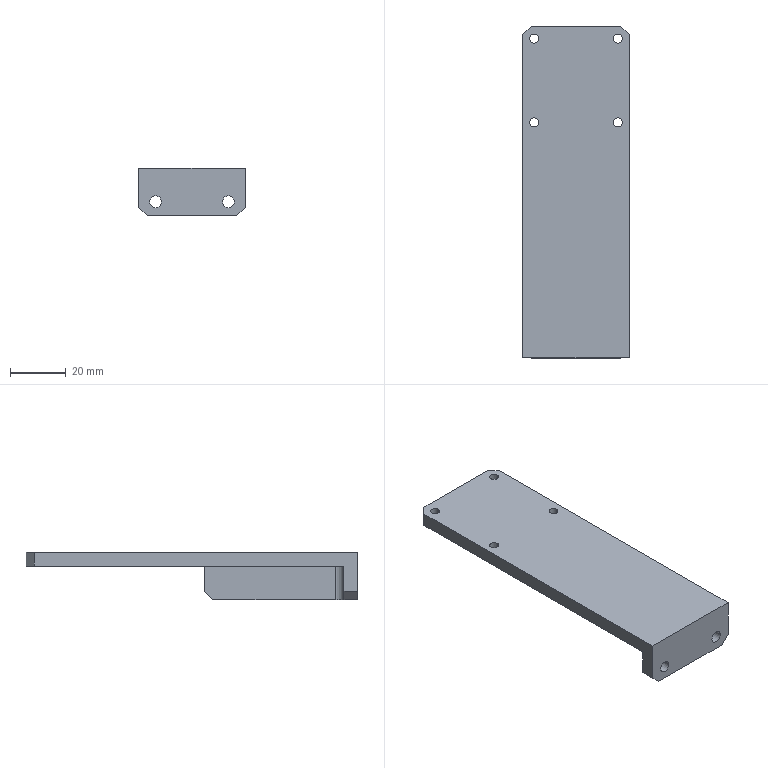NC program | NX | posted with a generic post | part box 38.1 x 118.8 x 17 mm
Whole program:
N10 G17 G21 G94 G90
(FLOOR_WALL_COPY , TOOL : D80)
N12 T19 M6
N14 G54
N16 G17 G0 G90 X-108.4 Y0. S6500 M3
N18 G43 Z30. H19
N20 Z3.
N22 G94 G1 Z0. F1500.
N24 X-103.4
N26 X103.4
N28 X108.4
N30 Z3.
N32 G0 Z30.
N34 M5
(DRILLING_COPY_1 , TOOL : D6A45)
N36 T01 M6
N38 G54
N40 G17 G0 G90 X24.9 Y15. S5000 M3
N42 G43 Z30. H1
N44 G94 G81 G98 Z-1. F350. R3.
N46 X54.9
N48 Y-15.
N50 X24.9
N52 G80
N54 G0 X24.9 Y-15. Z30.
N56 M5
(DRILLING_COPY_1_COPY_1 , TOOL : 3.2ZT)
N58 T03 M6
N60 G54
N62 G17 G0 G90 X24.9 Y15. S2000 M3
N64 G43 Z30. H3
N66 G94 G83 G98 Z-7.461 F180. Q2. R3.
N68 X54.9
N70 Y-15.
N72 X24.9
N74 G80
N76 G0 X24.9 Y-15. Z30.
N78 M5
(ADAPTIVE_MILLING , TOOL : D10)
N80 T15 M6
N82 G54
N84 G17 G0 G90 X0.038 Y30.759 S9500 M3
N86 G43 Z30. H15
N88 Z-14.
N90 G94 G1 Z-17. F1000.
N92 X-0.241 Y29.978 F3000.
N94 X-0.498 Y29.19
N96 G3 X0.038 Y28.112 R1.017
N98 X3.102 Y27.351 R8.28
N100 X12.969 Y27.069 R111.643
N102 G1 X15.219 Y27.064
N104 X19.094 Y27.061
N106 X32.719 Y27.06
N108 X60.344
N110 X60.594 Y27.055
N112 X60.719 Y27.046
N114 G2 X64.982 Y24.28 R5.993
N116 X66.931 Y18.661 R13.127
N118 X67.368 Y9.428 R74.333
N120 G1 X67.376 Y8.053
N122 X67.382 Y6.178
N124 X67.386 Y3.428
N126 X67.388 Y-2.072
N128 Y-20.072
N130 X67.386 Y-20.197
N132 G2 X64.882 Y-24.473 R5.736
N134 X59.312 Y-26.542 R12.477
N136 X50.457 Y-27.012 R65.248
N138 G1 X49.082 Y-27.022
N140 X47.582 Y-27.029
N142 X45.457 Y-27.034
N144 X42.082 Y-27.037
N146 X32.582 Y-27.038
N148 X-60.418
N150 G2 X-64.585 Y-24.819 R5.588
N152 X-66.807 Y-19.448 R11.664
N154 X-67.341 Y-11.85 R49.288
N156 G1 X-67.353 Y-10.975
N158 X-67.363 Y-9.975
N160 X-67.372 Y-8.725
N162 X-67.379 Y-7.1
N164 X-67.384 Y-4.85
N166 X-67.387 Y-1.1
N168 X-67.388 Y10.9
N170 Y20.025
N172 X-67.387 Y20.15
N174 X-67.382 Y20.275
N176 X-67.374 Y20.399
N178 G2 X-64.602 Y24.658 R5.958
N180 X-58.977 Y26.588 R13.219
N182 X-50.368 Y27.013 R69.988
N184 G1 X-49.118 Y27.021
N186 X-47.493 Y27.029
N188 X-45.243 Y27.034
N190 X-41.618 Y27.037
N192 X-30.618 Y27.038
N194 X-3.743
N196 G2 X1.729 Y26.518 R60.908
N198 G3 X13.217 Y26.09 R124.4
N200 G1 X14.967 Y26.082
N202 X17.092 Y26.077
N204 X20.467 Y26.073
N206 X27.217 Y26.071
N208 X57.217 Y26.07
N210 X57.467 Y26.068
N212 G2 X63.753 Y22.33 R7.674
N214 X65.873 Y15.977 R15.701
N216 X66.349 Y6.37 R79.223
N218 G1 X66.358 Y5.12
N220 X66.366 Y3.495
N222 X66.372 Y1.245
N224 X66.375 Y-2.13
N226 X66.377 Y-9.63
N228 Y-17.005
N230 G2 X62.752 Y-23.349 R7.595
N232 X56.539 Y-25.491 R15.229
N234 X46.81 Y-25.998 R75.518
N236 G1 X45.435 Y-26.008
N238 X43.935 Y-26.015
N240 X41.81 Y-26.021
N242 X38.81 Y-26.025
N244 X32.435 Y-26.027
N246 X-57.315
N248 G2 X-63.675 Y-22.429 R7.603
N250 X-65.867 Y-15.974 R15.279
N252 X-66.345 Y-6.743 R74.856
N254 G1 X-66.355 Y-5.618
N256 X-66.363 Y-4.118
N258 X-66.369 Y-2.243
N260 X-66.374 Y0.507
N262 X-66.377 Y5.382
N264 Y16.882
N266 G2 X-62.743 Y23.346 R7.598
N268 X-56.283 Y25.527 R15.448
N270 X-46.926 Y25.997 R78.149
N272 G1 X-45.676 Y26.007
N274 X-44.301 Y26.014
N276 X-42.551 Y26.02
N278 X-39.801 Y26.024
N280 X-34.801 Y26.027
N282 X-6.176
N284 G2 X1.431 Y25.542 R94.226
N286 G3 X16.545 Y25.095 R192.713
N288 G1 X18.795 Y25.088
N290 X22.045 Y25.084
N292 X27.92 Y25.082
N294 X54.295 Y25.081
N296 X54.67 Y25.079
N298 X54.92 Y25.076
N300 G2 X62.852 Y20.266 R8.971
N302 G3 X63.887 Y18.561 R8.559
N304 G2 X64.702 Y15.593 R8.871
N306 X65.319 Y5.495 R74.892
N308 G1 X65.332 Y4.37
N310 X65.341 Y3.246
N312 X65.35 Y1.746
N314 X65.357 Y-0.129
N316 X65.362 Y-2.754
N318 X65.365 Y-7.004
N320 G2 X65.328 Y-15.378 R300.794
N322 X60.743 Y-22.413 R8.874
N324 G3 X58.911 Y-23.537 R10.258
N326 G2 X55.944 Y-24.353 R8.925
N328 X45.47 Y-24.973 R78.124
N330 G1 X44.22 Y-24.986
N332 X42.97 Y-24.996
N334 X41.47 Y-25.003
N336 X39.345 Y-25.009
N338 X36.22 Y-25.014
N340 X30.345 Y-25.016
N342 X-54.655 Y-25.017
N344 X-55.03 Y-25.012
N346 X-55.155 Y-25.009
N348 X-55.404 Y-25.
N350 X-55.529 Y-24.993
N352 G2 X-58.795 Y-24.212 R11.41
N354 X-60.797 Y-23.998 R12.163
N356 X-63.887 Y-21.561 R5.458
N358 X-64.545 Y-19.084 R5.984
N360 X-65.342 Y-3.74 R126.963
N362 G1 X-65.351 Y-2.115
N364 X-65.358 Y0.01
N366 X-65.363 Y3.01
N368 X-65.366 Y8.01
N370 Y14.26
N372 X-65.363 Y14.635
N374 G2 X-64.572 Y18.401 R9.73
N376 X-64.348 Y20.447 R14.412
N378 X-61.911 Y23.537 R5.458
N380 X-59.434 Y24.195 R5.984
N382 X-44.84 Y24.986 R120.72
N384 G1 X-43.34 Y24.996
N386 X-41.465 Y25.005
N388 X-39.09 Y25.01
N390 X-35.465 Y25.015
N392 X-28.09 Y25.016
N394 X-7.84 Y25.017
N396 G2 X0.896 Y24.573 R122.606
N398 G3 X9.117 Y24.2 R216.611
N400 G1 X56.365
N402 X56.434 Y24.195
N404 G2 X60.014 Y22.713 R5.569
N406 G1 X60.066 Y22.667
N408 X63.017 Y19.716
N410 X63.063 Y19.664
N412 X63.443 Y19.168
N414 X63.676 Y18.872
N416 X63.887 Y18.561
N418 X64.348 Y17.447
N420 X64.384 Y17.314
N422 X64.545 Y16.084
N424 X64.55 Y16.015
N426 Y-16.015
N428 X64.545 Y-16.084
N430 G2 X63.063 Y-19.664 R5.569
N432 G1 X63.017 Y-19.716
N434 X60.066 Y-22.667
N436 X60.014 Y-22.713
N438 X59.617 Y-23.017
N440 X59.273 Y-23.289
N442 X58.911 Y-23.537
N444 X57.797 Y-23.998
N446 X57.664 Y-24.034
N448 X56.434 Y-24.195
N450 X56.365 Y-24.2
N452 X-58.885
N454 G2 X-62.03 Y-23.468 R6.018
N456 X-64.384 Y-20.314 R5.458
N458 G1 X-64.545 Y-19.084
N460 X-64.55 Y-19.015
N462 Y18.61
N464 G2 X-63.818 Y21.68 R5.969
N466 X-60.664 Y24.034 R5.458
N468 G1 X-59.434 Y24.195
N470 X-59.365 Y24.2
N472 X9.135
N474 G3 X10.132 Y25.05 R1.016
N476 G1 X10.383 Y26.621
N478 Z-14.
N480 G0 Z30.
N482 M5
(ZLEVEL_PROFILE_COPY_1_COPY_COPY_1 , TOOL : D10JING)
N484 T14 M6
N486 G54
N488 G17 G0 G90 X-61.022 Y25.859 S9500 M3
N490 G43 Z30. H14
N492 Z-16.
N494 G94 G1 Z-17. F1000.
N496 X-60.266 Y24.55
N498 G3 X-59.4 Y24.05 R1.
N500 G1 X56.4 F1200.
N502 G2 X59.936 Y22.586 R5.
N504 G1 X62.936 Y19.586
N506 G2 X64.4 Y16.05 R5.
N508 G1 Y-16.05
N510 G2 X62.936 Y-19.586 R5.
N512 G1 X59.936 Y-22.586
N514 G2 X56.4 Y-24.05 R5.
N516 G1 X-59.4
N518 G2 X-64.4 Y-19.05 R5.
N520 G1 Y19.05
N522 G2 X-59.4 Y24.05 R5.
N524 G3 X-58.534 Y24.55 R1.
N526 G1 X-57.668 Y26.05
N528 Z-16.
N530 G0 Z30.
N532 M5
(PLANAR_MILL_COPY_COPY_COPY_COPY_COPY_COPY_1_COPY_1 , TOOL : D6A45)
N534 T01 M6
N536 G54
N538 G17 G0 G90 X55.333 Y15.45 S9500 M3
N540 G43 Z30. H1
N542 Z0.5
N544 G94 G1 Z-1. F1250.
N546 G3 X54.9 Y15.7 R0.5
N548 X54.2 Y15. R0.7
N550 X54.9 Y15.7 R-0.7
N552 X54.467 Y15.45 R0.5
N554 G1 Z0.5
N556 G0 Z30.
N558 X25.333
N560 Z0.5
N562 G1 Z-1.
N564 G3 X24.9 Y15.7 R0.5
N566 X24.2 Y15. R0.7
N568 X24.9 Y15.7 R-0.7
N570 X24.467 Y15.45 R0.5
N572 G1 Z0.5
N574 G0 Z30.
N576 X-2.366 Y20.45
N578 Z0.5
N580 G1 Z-1.
N582 G3 X-1.5 Y19.95 R1.
N584 G1 X56.4
N586 G2 X57.036 Y19.686 R0.9
N588 G1 X60.036 Y16.686
N590 G2 X60.3 Y16.05 R0.9
N592 G1 Y-16.05
N594 G2 X60.036 Y-16.686 R0.9
N596 G1 X57.036 Y-19.686
N598 G2 X56.4 Y-19.95 R0.9
N600 G1 X-59.4
N602 G2 X-60.3 Y-19.05 R0.9
N604 G1 Y19.05
N606 G2 X-59.4 Y19.95 R0.9
N608 G1 X-1.5
N610 G3 X-0.634 Y20.45 R1.
N612 G1 Z0.5
N614 G0 Z30.
N616 X24.467 Y-15.45
N618 Z0.5
N620 G1 Z-1.
N622 G3 X24.9 Y-15.7 R0.5
N624 X25.6 Y-15. R0.7
N626 X24.9 Y-15.7 R-0.7
N628 X25.333 Y-15.45 R0.5
N630 G1 Z0.5
N632 G0 Z30.
N634 X54.467
N636 Z0.5
N638 G1 Z-1.
N640 G3 X54.9 Y-15.7 R0.5
N642 X55.6 Y-15. R0.7
N644 X54.9 Y-15.7 R-0.7
N646 X55.333 Y-15.45 R0.5
N648 G1 Z0.5
N650 G0 Z30.
N652 M5
N654 M2